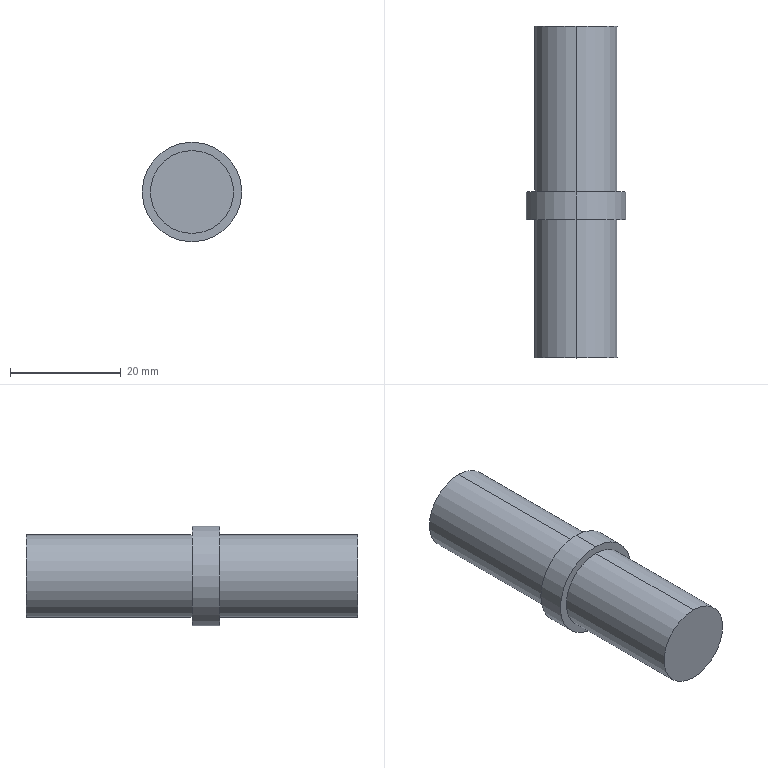Part | SolidWorks | features BaseBody 1 | 1 solid | 10 faces | box 18 x 60 x 18 mm | volume 10992 mm3 | cylinder 6 | plane 4 | commonest cylinder face diameters 15 x4 18 x2
STEP:
#1=CARTESIAN_POINT('',(0.,25.,7.5));
#2=VERTEX_POINT('',#1);
#3=CARTESIAN_POINT('',(0.,0.,7.5));
#4=VERTEX_POINT('',#3);
#5=CARTESIAN_POINT('',(0.,0.,7.5));
#6=DIRECTION('',(0.,-1.,0.));
#7=VECTOR('',#6,1000.);
#8=LINE('',#5,#7);
#9=EDGE_CURVE('',#2,#4,#8,.T.);
#10=ORIENTED_EDGE('',*,*,#9,.F.);
#11=CARTESIAN_POINT('',(0.,25.,-7.5));
#12=VERTEX_POINT('',#11);
#13=CARTESIAN_POINT('',(0.,25.,0.));
#14=DIRECTION('',(0.,-1.,0.));
#15=DIRECTION('',(0.,0.,-1.));
#16=AXIS2_PLACEMENT_3D('',#13,#14,#15);
#17=CIRCLE('',#16,7.5);
#18=EDGE_CURVE('',#2,#12,#17,.T.);
#19=ORIENTED_EDGE('',*,*,#18,.T.);
#20=CARTESIAN_POINT('',(0.,0.,-7.5));
#21=VERTEX_POINT('',#20);
#22=CARTESIAN_POINT('',(0.,0.,-7.5));
#23=DIRECTION('',(0.,-1.,0.));
#24=VECTOR('',#23,1000.);
#25=LINE('',#22,#24);
#26=EDGE_CURVE('',#12,#21,#25,.T.);
#27=ORIENTED_EDGE('',*,*,#26,.T.);
#28=CARTESIAN_POINT('',(0.,0.,0.));
#29=DIRECTION('',(0.,-1.,0.));
#30=DIRECTION('',(0.,0.,-1.));
#31=AXIS2_PLACEMENT_3D('',#28,#29,#30);
#32=CIRCLE('',#31,7.5);
#33=EDGE_CURVE('',#4,#21,#32,.T.);
#34=ORIENTED_EDGE('',*,*,#33,.F.);
#35=EDGE_LOOP('',(#10,#19,#27,#34));
#36=FACE_OUTER_BOUND('',#35,.T.);
#37=CARTESIAN_POINT('',(0.,0.,0.));
#38=DIRECTION('',(0.,-1.,0.));
#39=DIRECTION('',(0.,0.,-1.));
#40=AXIS2_PLACEMENT_3D('',#37,#38,#39);
#41=CYLINDRICAL_SURFACE('',#40,7.5);
#42=ADVANCED_FACE('',(#36),#41,.T.);
#43=CARTESIAN_POINT('',(0.,25.,0.));
#44=DIRECTION('',(0.,-1.,0.));
#45=DIRECTION('',(0.,0.,-1.));
#46=AXIS2_PLACEMENT_3D('',#43,#44,#45);
#47=CIRCLE('',#46,7.5);
#48=EDGE_CURVE('',#12,#2,#47,.T.);
#49=ORIENTED_EDGE('',*,*,#48,.F.);
#50=ORIENTED_EDGE('',*,*,#18,.F.);
#51=EDGE_LOOP('',(#49,#50));
#52=FACE_BOUND('',#51,.T.);
#53=CARTESIAN_POINT('',(0.,25.,-9.));
#54=VERTEX_POINT('',#53);
#55=CARTESIAN_POINT('',(0.,25.,9.));
#56=VERTEX_POINT('',#55);
#57=CARTESIAN_POINT('',(0.,25.,0.));
#58=DIRECTION('',(0.,-1.,0.));
#59=DIRECTION('',(0.,0.,-1.));
#60=AXIS2_PLACEMENT_3D('',#57,#58,#59);
#61=CIRCLE('',#60,9.);
#62=EDGE_CURVE('',#54,#56,#61,.T.);
#63=ORIENTED_EDGE('',*,*,#62,.T.);
#64=CARTESIAN_POINT('',(0.,25.,0.));
#65=DIRECTION('',(0.,-1.,0.));
#66=DIRECTION('',(0.,0.,-1.));
#67=AXIS2_PLACEMENT_3D('',#64,#65,#66);
#68=CIRCLE('',#67,9.);
#69=EDGE_CURVE('',#56,#54,#68,.T.);
#70=ORIENTED_EDGE('',*,*,#69,.T.);
#71=EDGE_LOOP('',(#63,#70));
#72=FACE_OUTER_BOUND('',#71,.T.);
#73=CARTESIAN_POINT('',(-9.,25.,0.));
#74=DIRECTION('',(0.,1.,0.));
#75=DIRECTION('',(1.,0.,0.));
#76=AXIS2_PLACEMENT_3D('',#73,#74,#75);
#77=PLANE('',#76);
#78=ADVANCED_FACE('',(#52,#72),#77,.F.);
#79=CARTESIAN_POINT('',(0.,30.,9.));
#80=VERTEX_POINT('',#79);
#81=CARTESIAN_POINT('',(0.,0.,9.));
#82=DIRECTION('',(0.,-1.,0.));
#83=VECTOR('',#82,1000.);
#84=LINE('',#81,#83);
#85=EDGE_CURVE('',#80,#56,#84,.T.);
#86=ORIENTED_EDGE('',*,*,#85,.F.);
#87=CARTESIAN_POINT('',(0.,30.,-9.));
#88=VERTEX_POINT('',#87);
#89=CARTESIAN_POINT('',(0.,30.,0.));
#90=DIRECTION('',(0.,-1.,0.));
#91=DIRECTION('',(0.,0.,-1.));
#92=AXIS2_PLACEMENT_3D('',#89,#90,#91);
#93=CIRCLE('',#92,9.);
#94=EDGE_CURVE('',#80,#88,#93,.T.);
#95=ORIENTED_EDGE('',*,*,#94,.T.);
#96=CARTESIAN_POINT('',(0.,0.,-9.));
#97=DIRECTION('',(0.,-1.,0.));
#98=VECTOR('',#97,1000.);
#99=LINE('',#96,#98);
#100=EDGE_CURVE('',#88,#54,#99,.T.);
#101=ORIENTED_EDGE('',*,*,#100,.T.);
#102=ORIENTED_EDGE('',*,*,#69,.F.);
#103=EDGE_LOOP('',(#86,#95,#101,#102));
#104=FACE_OUTER_BOUND('',#103,.T.);
#105=CARTESIAN_POINT('',(0.,0.,0.));
#106=DIRECTION('',(0.,-1.,0.));
#107=DIRECTION('',(0.,0.,-1.));
#108=AXIS2_PLACEMENT_3D('',#105,#106,#107);
#109=CYLINDRICAL_SURFACE('',#108,9.);
#110=ADVANCED_FACE('',(#104),#109,.T.);
#111=CARTESIAN_POINT('',(0.,30.,-7.5));
#112=VERTEX_POINT('',#111);
#113=CARTESIAN_POINT('',(0.,30.,7.5));
#114=VERTEX_POINT('',#113);
#115=CARTESIAN_POINT('',(0.,30.,0.));
#116=DIRECTION('',(0.,-1.,0.));
#117=DIRECTION('',(0.,0.,-1.));
#118=AXIS2_PLACEMENT_3D('',#115,#116,#117);
#119=CIRCLE('',#118,7.5);
#120=EDGE_CURVE('',#112,#114,#119,.T.);
#121=ORIENTED_EDGE('',*,*,#120,.T.);
#122=CARTESIAN_POINT('',(0.,30.,0.));
#123=DIRECTION('',(0.,-1.,0.));
#124=DIRECTION('',(0.,0.,-1.));
#125=AXIS2_PLACEMENT_3D('',#122,#123,#124);
#126=CIRCLE('',#125,7.5);
#127=EDGE_CURVE('',#114,#112,#126,.T.);
#128=ORIENTED_EDGE('',*,*,#127,.T.);
#129=EDGE_LOOP('',(#121,#128));
#130=FACE_BOUND('',#129,.T.);
#131=CARTESIAN_POINT('',(0.,30.,0.));
#132=DIRECTION('',(0.,-1.,0.));
#133=DIRECTION('',(0.,0.,-1.));
#134=AXIS2_PLACEMENT_3D('',#131,#132,#133);
#135=CIRCLE('',#134,9.);
#136=EDGE_CURVE('',#88,#80,#135,.T.);
#137=ORIENTED_EDGE('',*,*,#136,.F.);
#138=ORIENTED_EDGE('',*,*,#94,.F.);
#139=EDGE_LOOP('',(#137,#138));
#140=FACE_OUTER_BOUND('',#139,.T.);
#141=CARTESIAN_POINT('',(-7.5,30.,0.));
#142=DIRECTION('',(0.,-1.,0.));
#143=DIRECTION('',(0.,0.,-1.));
#144=AXIS2_PLACEMENT_3D('',#141,#142,#143);
#145=PLANE('',#144);
#146=ADVANCED_FACE('',(#130,#140),#145,.F.);
#147=CARTESIAN_POINT('',(0.,60.,7.5));
#148=VERTEX_POINT('',#147);
#149=CARTESIAN_POINT('',(0.,0.,7.5));
#150=DIRECTION('',(0.,-1.,0.));
#151=VECTOR('',#150,1000.);
#152=LINE('',#149,#151);
#153=EDGE_CURVE('',#148,#114,#152,.T.);
#154=ORIENTED_EDGE('',*,*,#153,.F.);
#155=CARTESIAN_POINT('',(0.,60.,-7.5));
#156=VERTEX_POINT('',#155);
#157=CARTESIAN_POINT('',(0.,60.,0.));
#158=DIRECTION('',(0.,-1.,0.));
#159=DIRECTION('',(0.,0.,-1.));
#160=AXIS2_PLACEMENT_3D('',#157,#158,#159);
#161=CIRCLE('',#160,7.5);
#162=EDGE_CURVE('',#148,#156,#161,.T.);
#163=ORIENTED_EDGE('',*,*,#162,.T.);
#164=CARTESIAN_POINT('',(0.,0.,-7.5));
#165=DIRECTION('',(0.,-1.,0.));
#166=VECTOR('',#165,1000.);
#167=LINE('',#164,#166);
#168=EDGE_CURVE('',#156,#112,#167,.T.);
#169=ORIENTED_EDGE('',*,*,#168,.T.);
#170=ORIENTED_EDGE('',*,*,#127,.F.);
#171=EDGE_LOOP('',(#154,#163,#169,#170));
#172=FACE_OUTER_BOUND('',#171,.T.);
#173=CARTESIAN_POINT('',(0.,0.,0.));
#174=DIRECTION('',(0.,-1.,0.));
#175=DIRECTION('',(0.,0.,-1.));
#176=AXIS2_PLACEMENT_3D('',#173,#174,#175);
#177=CYLINDRICAL_SURFACE('',#176,7.5);
#178=ADVANCED_FACE('',(#172),#177,.T.);
#179=CARTESIAN_POINT('',(0.,60.,0.));
#180=DIRECTION('',(0.,-1.,0.));
#181=DIRECTION('',(0.,0.,-1.));
#182=AXIS2_PLACEMENT_3D('',#179,#180,#181);
#183=CIRCLE('',#182,7.5);
#184=EDGE_CURVE('',#156,#148,#183,.T.);
#185=ORIENTED_EDGE('',*,*,#184,.F.);
#186=ORIENTED_EDGE('',*,*,#162,.F.);
#187=EDGE_LOOP('',(#185,#186));
#188=FACE_OUTER_BOUND('',#187,.T.);
#189=CARTESIAN_POINT('',(0.,60.,0.));
#190=DIRECTION('',(0.,-1.,0.));
#191=DIRECTION('',(0.,0.,-1.));
#192=AXIS2_PLACEMENT_3D('',#189,#190,#191);
#193=PLANE('',#192);
#194=ADVANCED_FACE('',(#188),#193,.F.);
#195=CARTESIAN_POINT('',(0.,0.,0.));
#196=DIRECTION('',(0.,-1.,0.));
#197=DIRECTION('',(0.,0.,-1.));
#198=AXIS2_PLACEMENT_3D('',#195,#196,#197);
#199=CIRCLE('',#198,7.5);
#200=EDGE_CURVE('',#21,#4,#199,.T.);
#201=ORIENTED_EDGE('',*,*,#200,.T.);
#202=ORIENTED_EDGE('',*,*,#33,.T.);
#203=EDGE_LOOP('',(#201,#202));
#204=FACE_OUTER_BOUND('',#203,.T.);
#205=CARTESIAN_POINT('',(-7.5,0.,0.));
#206=DIRECTION('',(0.,1.,0.));
#207=DIRECTION('',(1.,0.,0.));
#208=AXIS2_PLACEMENT_3D('',#205,#206,#207);
#209=PLANE('',#208);
#210=ADVANCED_FACE('',(#204),#209,.F.);
#211=ORIENTED_EDGE('',*,*,#184,.T.);
#212=ORIENTED_EDGE('',*,*,#153,.T.);
#213=ORIENTED_EDGE('',*,*,#120,.F.);
#214=ORIENTED_EDGE('',*,*,#168,.F.);
#215=EDGE_LOOP('',(#211,#212,#213,#214));
#216=FACE_OUTER_BOUND('',#215,.T.);
#217=CARTESIAN_POINT('',(0.,0.,0.));
#218=DIRECTION('',(0.,-1.,0.));
#219=DIRECTION('',(0.,0.,-1.));
#220=AXIS2_PLACEMENT_3D('',#217,#218,#219);
#221=CYLINDRICAL_SURFACE('',#220,7.5);
#222=ADVANCED_FACE('',(#216),#221,.T.);
#223=ORIENTED_EDGE('',*,*,#136,.T.);
#224=ORIENTED_EDGE('',*,*,#85,.T.);
#225=ORIENTED_EDGE('',*,*,#62,.F.);
#226=ORIENTED_EDGE('',*,*,#100,.F.);
#227=EDGE_LOOP('',(#223,#224,#225,#226));
#228=FACE_OUTER_BOUND('',#227,.T.);
#229=CARTESIAN_POINT('',(0.,0.,0.));
#230=DIRECTION('',(0.,-1.,0.));
#231=DIRECTION('',(0.,0.,-1.));
#232=AXIS2_PLACEMENT_3D('',#229,#230,#231);
#233=CYLINDRICAL_SURFACE('',#232,9.);
#234=ADVANCED_FACE('',(#228),#233,.T.);
#235=ORIENTED_EDGE('',*,*,#48,.T.);
#236=ORIENTED_EDGE('',*,*,#9,.T.);
#237=ORIENTED_EDGE('',*,*,#200,.F.);
#238=ORIENTED_EDGE('',*,*,#26,.F.);
#239=EDGE_LOOP('',(#235,#236,#237,#238));
#240=FACE_OUTER_BOUND('',#239,.T.);
#241=CARTESIAN_POINT('',(0.,0.,0.));
#242=DIRECTION('',(0.,-1.,0.));
#243=DIRECTION('',(0.,0.,-1.));
#244=AXIS2_PLACEMENT_3D('',#241,#242,#243);
#245=CYLINDRICAL_SURFACE('',#244,7.5);
#246=ADVANCED_FACE('',(#240),#245,.T.);
#247=CLOSED_SHELL('',(#42,#78,#110,#146,#178,#194,#210,#222,#234,#246));
#248=MANIFOLD_SOLID_BREP('',#247);
#249=CARTESIAN_POINT('',(0.,0.,0.));
#250=DIRECTION('',(0.,0.,1.));
#251=DIRECTION('',(1.,0.,0.));
#252=AXIS2_PLACEMENT_3D('',#249,#250,#251);
#253=(LENGTH_UNIT()NAMED_UNIT(*)SI_UNIT(.MILLI.,.METRE.));
#254=UNCERTAINTY_MEASURE_WITH_UNIT(LENGTH_MEASURE(0.00001),#253,'','');
#255=(NAMED_UNIT(*)PLANE_ANGLE_UNIT()SI_UNIT($,.RADIAN.));
#256=(NAMED_UNIT(*)SI_UNIT($,.STERADIAN.)SOLID_ANGLE_UNIT());
#257=(GEOMETRIC_REPRESENTATION_CONTEXT(3)GLOBAL_UNCERTAINTY_ASSIGNED_CONTEXT((#254))GLOBAL_UNIT_ASSIGNED_CONTEXT((#253,#255,#256))REPRESENTATION_CONTEXT('',''));
#258=ADVANCED_BREP_SHAPE_REPRESENTATION('',(#248,#252),#257);